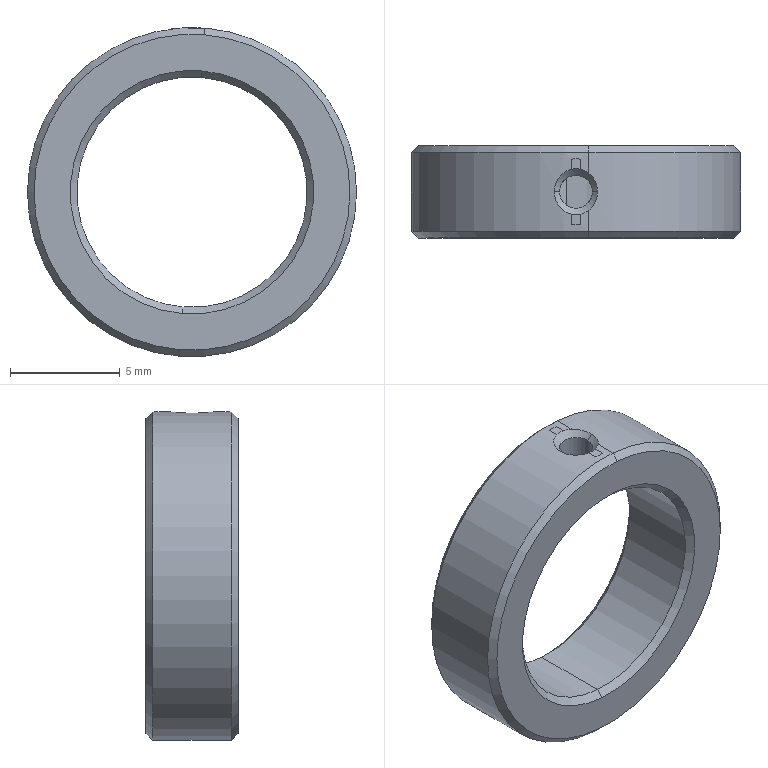Part | STEP file | 2026.6.15-Main Assembly图.sldasm-Part-197 | 1 solid | 20 faces | box 15 x 4.2 x 15 mm | volume 367.131 mm3 | cone 10 | cylinder 6 | plane 4 | commonest cylinder face diameters 1.5 x2 10.5 x2 15 x2
STEP:
#1=CARTESIAN_POINT('',(-1629.724,1422.164,3402.553));
#2=VERTEX_POINT('',#1);
#3=CARTESIAN_POINT('',(-1629.7,1422.464,3402.853));
#4=VERTEX_POINT('',#3);
#5=CARTESIAN_POINT('',(-1629.724,1422.164,3402.553));
#6=DIRECTION('',(0.0555,0.7071,0.7049));
#7=VECTOR('',#6,1000.);
#8=LINE('',#5,#7);
#9=EDGE_CURVE('',#2,#4,#8,.T.);
#10=ORIENTED_EDGE('',*,*,#9,.T.);
#11=CARTESIAN_POINT('',(-1628.876,1422.464,3413.32));
#12=VERTEX_POINT('',#11);
#13=CARTESIAN_POINT('',(-1629.288,1422.464,3408.086));
#14=DIRECTION('',(0.,1.,0.));
#15=DIRECTION('',(0.0785,0.,0.9969));
#16=AXIS2_PLACEMENT_3D('',#13,#14,#15);
#17=CIRCLE('',#16,5.25);
#18=EDGE_CURVE('',#4,#12,#17,.T.);
#19=ORIENTED_EDGE('',*,*,#18,.T.);
#20=CARTESIAN_POINT('',(-1628.853,1422.164,3413.619));
#21=VERTEX_POINT('',#20);
#22=CARTESIAN_POINT('',(-1628.853,1422.164,3413.619));
#23=DIRECTION('',(-0.0555,0.7071,-0.7049));
#24=VECTOR('',#23,1000.);
#25=LINE('',#22,#24);
#26=EDGE_CURVE('',#21,#12,#25,.T.);
#27=ORIENTED_EDGE('',*,*,#26,.F.);
#28=CARTESIAN_POINT('',(-1629.288,1422.164,3408.086));
#29=DIRECTION('',(0.,1.,0.));
#30=DIRECTION('',(0.0785,0.,0.9969));
#31=AXIS2_PLACEMENT_3D('',#28,#29,#30);
#32=CIRCLE('',#31,5.55);
#33=EDGE_CURVE('',#2,#21,#32,.T.);
#34=ORIENTED_EDGE('',*,*,#33,.F.);
#35=EDGE_LOOP('',(#10,#19,#27,#34));
#36=FACE_OUTER_BOUND('',#35,.T.);
#37=CARTESIAN_POINT('',(-1629.288,1422.164,3408.086));
#38=DIRECTION('',(0.,-1.,0.));
#39=DIRECTION('',(-0.0785,0.,-0.9969));
#40=AXIS2_PLACEMENT_3D('',#37,#38,#39);
#41=CONICAL_SURFACE('',#40,5.55,0.7854);
#42=ADVANCED_FACE('',(#36),#41,.F.);
#43=CARTESIAN_POINT('',(-1628.876,1426.064,3413.32));
#44=VERTEX_POINT('',#43);
#45=CARTESIAN_POINT('',(-1628.853,1426.364,3413.619));
#46=VERTEX_POINT('',#45);
#47=CARTESIAN_POINT('',(-1628.853,1426.364,3413.619));
#48=DIRECTION('',(0.0555,0.7071,0.7049));
#49=VECTOR('',#48,1000.);
#50=LINE('',#47,#49);
#51=EDGE_CURVE('',#44,#46,#50,.T.);
#52=ORIENTED_EDGE('',*,*,#51,.F.);
#53=CARTESIAN_POINT('',(-1629.7,1426.064,3402.853));
#54=VERTEX_POINT('',#53);
#55=CARTESIAN_POINT('',(-1629.288,1426.064,3408.086));
#56=DIRECTION('',(0.,-1.,0.));
#57=DIRECTION('',(0.0785,0.,0.9969));
#58=AXIS2_PLACEMENT_3D('',#55,#56,#57);
#59=CIRCLE('',#58,5.25);
#60=EDGE_CURVE('',#44,#54,#59,.T.);
#61=ORIENTED_EDGE('',*,*,#60,.T.);
#62=CARTESIAN_POINT('',(-1629.724,1426.364,3402.553));
#63=VERTEX_POINT('',#62);
#64=CARTESIAN_POINT('',(-1629.724,1426.364,3402.553));
#65=DIRECTION('',(-0.0555,0.7071,-0.7049));
#66=VECTOR('',#65,1000.);
#67=LINE('',#64,#66);
#68=EDGE_CURVE('',#54,#63,#67,.T.);
#69=ORIENTED_EDGE('',*,*,#68,.T.);
#70=CARTESIAN_POINT('',(-1629.288,1426.364,3408.086));
#71=DIRECTION('',(0.,1.,0.));
#72=DIRECTION('',(-0.0785,0.,-0.9969));
#73=AXIS2_PLACEMENT_3D('',#70,#71,#72);
#74=CIRCLE('',#73,5.55);
#75=EDGE_CURVE('',#63,#46,#74,.T.);
#76=ORIENTED_EDGE('',*,*,#75,.T.);
#77=EDGE_LOOP('',(#52,#61,#69,#76));
#78=FACE_OUTER_BOUND('',#77,.T.);
#79=CARTESIAN_POINT('',(-1629.288,1426.364,3408.086));
#80=DIRECTION('',(0.,1.,0.));
#81=DIRECTION('',(0.0785,0.,0.9969));
#82=AXIS2_PLACEMENT_3D('',#79,#80,#81);
#83=CONICAL_SURFACE('',#82,5.55,0.7854);
#84=ADVANCED_FACE('',(#78),#83,.F.);
#85=CARTESIAN_POINT('',(-1629.7,1404.739,3402.853));
#86=DIRECTION('',(0.,1.,0.));
#87=VECTOR('',#86,1000.);
#88=LINE('',#85,#87);
#89=EDGE_CURVE('',#4,#54,#88,.T.);
#90=ORIENTED_EDGE('',*,*,#89,.T.);
#91=ORIENTED_EDGE('',*,*,#60,.F.);
#92=CARTESIAN_POINT('',(-1628.876,1424.891,3413.32));
#93=VERTEX_POINT('',#92);
#94=CARTESIAN_POINT('',(-1628.876,1404.739,3413.32));
#95=DIRECTION('',(0.,1.,0.));
#96=VECTOR('',#95,1000.);
#97=LINE('',#94,#96);
#98=EDGE_CURVE('',#93,#44,#97,.T.);
#99=ORIENTED_EDGE('',*,*,#98,.F.);
#100=CARTESIAN_POINT('',(-1630.038,1424.264,3413.282));
#101=VERTEX_POINT('',#100);
#102=CARTESIAN_POINT('',(-1628.876,1424.891,3413.32));
#103=CARTESIAN_POINT('',(-1628.989,1424.965,3413.329));
#104=CARTESIAN_POINT('',(-1629.121,1425.008,3413.335));
#105=CARTESIAN_POINT('',(-1629.389,1425.019,3413.337));
#106=CARTESIAN_POINT('',(-1629.526,1424.988,3413.332));
#107=CARTESIAN_POINT('',(-1629.763,1424.861,3413.316));
#108=CARTESIAN_POINT('',(-1629.863,1424.765,3413.305));
#109=CARTESIAN_POINT('',(-1630.001,1424.534,3413.288));
#110=CARTESIAN_POINT('',(-1630.038,1424.4,3413.282));
#111=CARTESIAN_POINT('',(-1630.038,1424.264,3413.282));
#112=B_SPLINE_CURVE_WITH_KNOTS('',3,(#102,#103,#104,#105,#106,#107,#108,#109,#110,#111),.UNSPECIFIED.,.F.,.F.,(4,2,2,2,4),(0.,0.000402,0.000804,0.001206,0.001608),.UNSPECIFIED.);
#113=EDGE_CURVE('',#93,#101,#112,.T.);
#114=ORIENTED_EDGE('',*,*,#113,.T.);
#115=CARTESIAN_POINT('',(-1628.876,1423.638,3413.32));
#116=VERTEX_POINT('',#115);
#117=CARTESIAN_POINT('',(-1630.038,1424.264,3413.282));
#118=CARTESIAN_POINT('',(-1630.038,1424.128,3413.282));
#119=CARTESIAN_POINT('',(-1630.001,1423.995,3413.288));
#120=CARTESIAN_POINT('',(-1629.864,1423.765,3413.305));
#121=CARTESIAN_POINT('',(-1629.763,1423.668,3413.316));
#122=CARTESIAN_POINT('',(-1629.526,1423.541,3413.332));
#123=CARTESIAN_POINT('',(-1629.391,1423.509,3413.337));
#124=CARTESIAN_POINT('',(-1629.122,1423.521,3413.335));
#125=CARTESIAN_POINT('',(-1628.989,1423.563,3413.329));
#126=CARTESIAN_POINT('',(-1628.876,1423.638,3413.32));
#127=B_SPLINE_CURVE_WITH_KNOTS('',3,(#117,#118,#119,#120,#121,#122,#123,#124,#125,#126),.UNSPECIFIED.,.F.,.F.,(4,2,2,2,4),(0.,0.0004019,0.0008039,0.001206,0.001608),.UNSPECIFIED.);
#128=EDGE_CURVE('',#101,#116,#127,.T.);
#129=ORIENTED_EDGE('',*,*,#128,.T.);
#130=CARTESIAN_POINT('',(-1628.876,1404.739,3413.32));
#131=DIRECTION('',(0.,-1.,0.));
#132=VECTOR('',#131,1000.);
#133=LINE('',#130,#132);
#134=EDGE_CURVE('',#116,#12,#133,.T.);
#135=ORIENTED_EDGE('',*,*,#134,.T.);
#136=ORIENTED_EDGE('',*,*,#18,.F.);
#137=EDGE_LOOP('',(#90,#91,#99,#114,#129,#135,#136));
#138=FACE_OUTER_BOUND('',#137,.T.);
#139=CARTESIAN_POINT('',(-1629.288,1404.739,3408.086));
#140=DIRECTION('',(0.,-1.,0.));
#141=DIRECTION('',(-0.0785,0.,-0.9969));
#142=AXIS2_PLACEMENT_3D('',#139,#140,#141);
#143=CYLINDRICAL_SURFACE('',#142,5.25);
#144=ADVANCED_FACE('',(#138),#143,.F.);
#145=CARTESIAN_POINT('',(-1629.853,1422.164,3400.909));
#146=VERTEX_POINT('',#145);
#147=CARTESIAN_POINT('',(-1628.723,1422.164,3415.264));
#148=VERTEX_POINT('',#147);
#149=CARTESIAN_POINT('',(-1629.288,1422.164,3408.086));
#150=DIRECTION('',(0.,1.,0.));
#151=DIRECTION('',(-0.0785,0.,-0.9969));
#152=AXIS2_PLACEMENT_3D('',#149,#150,#151);
#153=CIRCLE('',#152,7.2);
#154=EDGE_CURVE('',#146,#148,#153,.T.);
#155=ORIENTED_EDGE('',*,*,#154,.F.);
#156=CARTESIAN_POINT('',(-1629.288,1422.164,3408.086));
#157=DIRECTION('',(0.,1.,0.));
#158=DIRECTION('',(-0.0785,0.,-0.9969));
#159=AXIS2_PLACEMENT_3D('',#156,#157,#158);
#160=CIRCLE('',#159,7.2);
#161=EDGE_CURVE('',#148,#146,#160,.T.);
#162=ORIENTED_EDGE('',*,*,#161,.F.);
#163=EDGE_LOOP('',(#155,#162));
#164=FACE_OUTER_BOUND('',#163,.T.);
#165=CARTESIAN_POINT('',(-1629.288,1422.164,3408.086));
#166=DIRECTION('',(0.,1.,0.));
#167=DIRECTION('',(0.0785,0.,0.9969));
#168=AXIS2_PLACEMENT_3D('',#165,#166,#167);
#169=CIRCLE('',#168,5.55);
#170=EDGE_CURVE('',#21,#2,#169,.T.);
#171=ORIENTED_EDGE('',*,*,#170,.T.);
#172=ORIENTED_EDGE('',*,*,#33,.T.);
#173=EDGE_LOOP('',(#171,#172));
#174=FACE_BOUND('',#173,.T.);
#175=CARTESIAN_POINT('',(-1629.288,1422.164,3408.086));
#176=DIRECTION('',(0.,-1.,0.));
#177=DIRECTION('',(0.,0.,-1.));
#178=AXIS2_PLACEMENT_3D('',#175,#176,#177);
#179=PLANE('',#178);
#180=ADVANCED_FACE('',(#164,#174),#179,.T.);
#181=CARTESIAN_POINT('',(-1628.723,1426.364,3415.264));
#182=VERTEX_POINT('',#181);
#183=CARTESIAN_POINT('',(-1629.853,1426.364,3400.909));
#184=VERTEX_POINT('',#183);
#185=CARTESIAN_POINT('',(-1629.288,1426.364,3408.086));
#186=DIRECTION('',(0.,-1.,0.));
#187=DIRECTION('',(0.0785,0.,0.9969));
#188=AXIS2_PLACEMENT_3D('',#185,#186,#187);
#189=CIRCLE('',#188,7.2);
#190=EDGE_CURVE('',#182,#184,#189,.T.);
#191=ORIENTED_EDGE('',*,*,#190,.F.);
#192=CARTESIAN_POINT('',(-1629.288,1426.364,3408.086));
#193=DIRECTION('',(0.,-1.,0.));
#194=DIRECTION('',(0.0785,0.,0.9969));
#195=AXIS2_PLACEMENT_3D('',#192,#193,#194);
#196=CIRCLE('',#195,7.2);
#197=EDGE_CURVE('',#184,#182,#196,.T.);
#198=ORIENTED_EDGE('',*,*,#197,.F.);
#199=EDGE_LOOP('',(#191,#198));
#200=FACE_OUTER_BOUND('',#199,.T.);
#201=ORIENTED_EDGE('',*,*,#75,.F.);
#202=CARTESIAN_POINT('',(-1629.288,1426.364,3408.086));
#203=DIRECTION('',(0.,1.,0.));
#204=DIRECTION('',(-0.0785,0.,-0.9969));
#205=AXIS2_PLACEMENT_3D('',#202,#203,#204);
#206=CIRCLE('',#205,5.55);
#207=EDGE_CURVE('',#46,#63,#206,.T.);
#208=ORIENTED_EDGE('',*,*,#207,.F.);
#209=EDGE_LOOP('',(#201,#208));
#210=FACE_BOUND('',#209,.T.);
#211=CARTESIAN_POINT('',(-1629.288,1426.364,3408.086));
#212=DIRECTION('',(0.,-1.,0.));
#213=DIRECTION('',(0.,0.,-1.));
#214=AXIS2_PLACEMENT_3D('',#211,#212,#213);
#215=PLANE('',#214);
#216=ADVANCED_FACE('',(#200,#210),#215,.F.);
#217=CARTESIAN_POINT('',(-1629.5,1425.29,3415.583));
#218=VERTEX_POINT('',#217);
#219=CARTESIAN_POINT('',(-1629.5,1425.749,3415.583));
#220=VERTEX_POINT('',#219);
#221=CARTESIAN_POINT('',(-1629.5,1426.364,3415.583));
#222=DIRECTION('',(0.,1.,0.));
#223=VECTOR('',#222,1000.);
#224=LINE('',#221,#223);
#225=EDGE_CURVE('',#218,#220,#224,.T.);
#226=ORIENTED_EDGE('',*,*,#225,.F.);
#227=CARTESIAN_POINT('',(-1629.076,1425.29,3415.583));
#228=VERTEX_POINT('',#227);
#229=CARTESIAN_POINT('',(-1629.288,1424.264,3415.583));
#230=DIRECTION('',(0.,0.,-1.));
#231=DIRECTION('',(1.,0.,0.));
#232=AXIS2_PLACEMENT_3D('',#229,#230,#231);
#233=CIRCLE('',#232,1.047);
#234=EDGE_CURVE('',#218,#228,#233,.T.);
#235=ORIENTED_EDGE('',*,*,#234,.T.);
#236=CARTESIAN_POINT('',(-1629.076,1425.749,3415.583));
#237=VERTEX_POINT('',#236);
#238=CARTESIAN_POINT('',(-1629.076,1426.364,3415.583));
#239=DIRECTION('',(0.,-1.,0.));
#240=VECTOR('',#239,1000.);
#241=LINE('',#238,#240);
#242=EDGE_CURVE('',#237,#228,#241,.T.);
#243=ORIENTED_EDGE('',*,*,#242,.F.);
#244=CARTESIAN_POINT('',(-1629.5,1425.749,3415.583));
#245=CARTESIAN_POINT('',(-1629.359,1425.769,3415.587));
#246=CARTESIAN_POINT('',(-1629.218,1425.769,3415.587));
#247=CARTESIAN_POINT('',(-1629.076,1425.749,3415.583));
#248=B_SPLINE_CURVE_WITH_KNOTS('',3,(#244,#245,#246,#247),.UNSPECIFIED.,.F.,.F.,(4,4),(0.,1.),.UNSPECIFIED.);
#249=EDGE_CURVE('',#220,#237,#248,.T.);
#250=ORIENTED_EDGE('',*,*,#249,.F.);
#251=EDGE_LOOP('',(#226,#235,#243,#250));
#252=FACE_OUTER_BOUND('',#251,.T.);
#253=CARTESIAN_POINT('',(-1629.288,1424.264,3415.583));
#254=DIRECTION('',(0.,0.,-1.));
#255=DIRECTION('',(1.,0.,0.));
#256=AXIS2_PLACEMENT_3D('',#253,#254,#255);
#257=PLANE('',#256);
#258=ADVANCED_FACE('',(#252),#257,.F.);
#259=CARTESIAN_POINT('',(-1629.5,1422.779,3415.583));
#260=VERTEX_POINT('',#259);
#261=CARTESIAN_POINT('',(-1629.5,1423.239,3415.583));
#262=VERTEX_POINT('',#261);
#263=CARTESIAN_POINT('',(-1629.5,1426.364,3415.583));
#264=DIRECTION('',(0.,1.,0.));
#265=VECTOR('',#264,1000.);
#266=LINE('',#263,#265);
#267=EDGE_CURVE('',#260,#262,#266,.T.);
#268=ORIENTED_EDGE('',*,*,#267,.F.);
#269=CARTESIAN_POINT('',(-1629.076,1422.779,3415.583));
#270=VERTEX_POINT('',#269);
#271=CARTESIAN_POINT('',(-1629.076,1422.779,3415.583));
#272=CARTESIAN_POINT('',(-1629.218,1422.759,3415.587));
#273=CARTESIAN_POINT('',(-1629.359,1422.759,3415.587));
#274=CARTESIAN_POINT('',(-1629.5,1422.779,3415.583));
#275=B_SPLINE_CURVE_WITH_KNOTS('',3,(#271,#272,#273,#274),.UNSPECIFIED.,.F.,.F.,(4,4),(0.,1.),.UNSPECIFIED.);
#276=EDGE_CURVE('',#270,#260,#275,.T.);
#277=ORIENTED_EDGE('',*,*,#276,.F.);
#278=CARTESIAN_POINT('',(-1629.076,1423.239,3415.583));
#279=VERTEX_POINT('',#278);
#280=CARTESIAN_POINT('',(-1629.076,1426.364,3415.583));
#281=DIRECTION('',(0.,-1.,0.));
#282=VECTOR('',#281,1000.);
#283=LINE('',#280,#282);
#284=EDGE_CURVE('',#279,#270,#283,.T.);
#285=ORIENTED_EDGE('',*,*,#284,.F.);
#286=CARTESIAN_POINT('',(-1629.288,1424.264,3415.583));
#287=DIRECTION('',(0.,0.,-1.));
#288=DIRECTION('',(1.,0.,0.));
#289=AXIS2_PLACEMENT_3D('',#286,#287,#288);
#290=CIRCLE('',#289,1.047);
#291=EDGE_CURVE('',#279,#262,#290,.T.);
#292=ORIENTED_EDGE('',*,*,#291,.T.);
#293=EDGE_LOOP('',(#268,#277,#285,#292));
#294=FACE_OUTER_BOUND('',#293,.T.);
#295=CARTESIAN_POINT('',(-1629.288,1424.264,3415.583));
#296=DIRECTION('',(0.,0.,-1.));
#297=DIRECTION('',(1.,0.,0.));
#298=AXIS2_PLACEMENT_3D('',#295,#296,#297);
#299=PLANE('',#298);
#300=ADVANCED_FACE('',(#294),#299,.F.);
#301=CARTESIAN_POINT('',(-1628.538,1424.264,3413.282));
#302=VERTEX_POINT('',#301);
#303=CARTESIAN_POINT('',(-1628.538,1424.264,3415.286));
#304=VERTEX_POINT('',#303);
#305=CARTESIAN_POINT('',(-1628.538,1424.264,3393.661));
#306=DIRECTION('',(0.,0.,1.));
#307=VECTOR('',#306,1000.);
#308=LINE('',#305,#307);
#309=EDGE_CURVE('',#302,#304,#308,.T.);
#310=ORIENTED_EDGE('',*,*,#309,.T.);
#311=CARTESIAN_POINT('',(-1630.038,1424.264,3415.286));
#312=VERTEX_POINT('',#311);
#313=CARTESIAN_POINT('',(-1629.288,1424.264,3415.286));
#314=DIRECTION('',(0.,0.,1.));
#315=DIRECTION('',(1.,0.,0.));
#316=AXIS2_PLACEMENT_3D('',#313,#314,#315);
#317=CIRCLE('',#316,0.75);
#318=EDGE_CURVE('',#304,#312,#317,.T.);
#319=ORIENTED_EDGE('',*,*,#318,.T.);
#320=CARTESIAN_POINT('',(-1630.038,1424.264,3393.661));
#321=DIRECTION('',(0.,0.,1.));
#322=VECTOR('',#321,1000.);
#323=LINE('',#320,#322);
#324=EDGE_CURVE('',#101,#312,#323,.T.);
#325=ORIENTED_EDGE('',*,*,#324,.F.);
#326=ORIENTED_EDGE('',*,*,#113,.F.);
#327=CARTESIAN_POINT('',(-1628.538,1424.264,3413.282));
#328=CARTESIAN_POINT('',(-1628.538,1424.389,3413.282));
#329=CARTESIAN_POINT('',(-1628.57,1424.512,3413.287));
#330=CARTESIAN_POINT('',(-1628.687,1424.729,3413.302));
#331=CARTESIAN_POINT('',(-1628.772,1424.822,3413.312));
#332=CARTESIAN_POINT('',(-1628.876,1424.891,3413.32));
#333=B_SPLINE_CURVE_WITH_KNOTS('',3,(#327,#328,#329,#330,#331,#332),.UNSPECIFIED.,.F.,.F.,(4,2,4),(0.,0.0003696,0.0007391),.UNSPECIFIED.);
#334=EDGE_CURVE('',#302,#93,#333,.T.);
#335=ORIENTED_EDGE('',*,*,#334,.F.);
#336=EDGE_LOOP('',(#310,#319,#325,#326,#335));
#337=FACE_OUTER_BOUND('',#336,.T.);
#338=CARTESIAN_POINT('',(-1629.288,1424.264,3393.661));
#339=DIRECTION('',(0.,0.,-1.));
#340=DIRECTION('',(1.,0.,0.));
#341=AXIS2_PLACEMENT_3D('',#338,#339,#340);
#342=CYLINDRICAL_SURFACE('',#341,0.75);
#343=ADVANCED_FACE('',(#337),#342,.F.);
#344=CARTESIAN_POINT('',(-1628.7,1422.464,3415.563));
#345=VERTEX_POINT('',#344);
#346=CARTESIAN_POINT('',(-1628.7,1422.464,3415.563));
#347=DIRECTION('',(0.0555,0.7071,0.7049));
#348=VECTOR('',#347,1000.);
#349=LINE('',#346,#348);
#350=EDGE_CURVE('',#148,#345,#349,.T.);
#351=ORIENTED_EDGE('',*,*,#350,.F.);
#352=ORIENTED_EDGE('',*,*,#161,.T.);
#353=CARTESIAN_POINT('',(-1629.877,1422.464,3400.609));
#354=VERTEX_POINT('',#353);
#355=CARTESIAN_POINT('',(-1629.877,1422.464,3400.609));
#356=DIRECTION('',(-0.0555,0.7071,-0.7049));
#357=VECTOR('',#356,1000.);
#358=LINE('',#355,#357);
#359=EDGE_CURVE('',#146,#354,#358,.T.);
#360=ORIENTED_EDGE('',*,*,#359,.T.);
#361=CARTESIAN_POINT('',(-1629.288,1422.464,3408.086));
#362=DIRECTION('',(0.,1.,0.));
#363=DIRECTION('',(-0.0785,0.,-0.9969));
#364=AXIS2_PLACEMENT_3D('',#361,#362,#363);
#365=CIRCLE('',#364,7.5);
#366=EDGE_CURVE('',#345,#354,#365,.T.);
#367=ORIENTED_EDGE('',*,*,#366,.F.);
#368=EDGE_LOOP('',(#351,#352,#360,#367));
#369=FACE_OUTER_BOUND('',#368,.T.);
#370=CARTESIAN_POINT('',(-1629.288,1422.464,3408.086));
#371=DIRECTION('',(0.,1.,0.));
#372=DIRECTION('',(0.0785,0.,0.9969));
#373=AXIS2_PLACEMENT_3D('',#370,#371,#372);
#374=CONICAL_SURFACE('',#373,7.5,0.7854);
#375=ADVANCED_FACE('',(#369),#374,.T.);
#376=CARTESIAN_POINT('',(-1629.877,1426.064,3400.609));
#377=VERTEX_POINT('',#376);
#378=CARTESIAN_POINT('',(-1629.877,1426.064,3400.609));
#379=DIRECTION('',(0.0555,0.7071,0.7049));
#380=VECTOR('',#379,1000.);
#381=LINE('',#378,#380);
#382=EDGE_CURVE('',#377,#184,#381,.T.);
#383=ORIENTED_EDGE('',*,*,#382,.T.);
#384=ORIENTED_EDGE('',*,*,#197,.T.);
#385=CARTESIAN_POINT('',(-1628.7,1426.064,3415.563));
#386=VERTEX_POINT('',#385);
#387=CARTESIAN_POINT('',(-1628.7,1426.064,3415.563));
#388=DIRECTION('',(-0.0555,0.7071,-0.7049));
#389=VECTOR('',#388,1000.);
#390=LINE('',#387,#389);
#391=EDGE_CURVE('',#386,#182,#390,.T.);
#392=ORIENTED_EDGE('',*,*,#391,.F.);
#393=CARTESIAN_POINT('',(-1629.288,1426.064,3408.086));
#394=DIRECTION('',(0.,-1.,0.));
#395=DIRECTION('',(-0.0785,0.,-0.9969));
#396=AXIS2_PLACEMENT_3D('',#393,#394,#395);
#397=CIRCLE('',#396,7.5);
#398=EDGE_CURVE('',#377,#386,#397,.T.);
#399=ORIENTED_EDGE('',*,*,#398,.F.);
#400=EDGE_LOOP('',(#383,#384,#392,#399));
#401=FACE_OUTER_BOUND('',#400,.T.);
#402=CARTESIAN_POINT('',(-1629.288,1426.064,3408.086));
#403=DIRECTION('',(0.,-1.,0.));
#404=DIRECTION('',(-0.0785,0.,-0.9969));
#405=AXIS2_PLACEMENT_3D('',#402,#403,#404);
#406=CONICAL_SURFACE('',#405,7.5,0.7854);
#407=ADVANCED_FACE('',(#401),#406,.T.);
#408=CARTESIAN_POINT('',(-1630.273,1424.264,3415.521));
#409=VERTEX_POINT('',#408);
#410=CARTESIAN_POINT('',(-1630.335,1424.264,3415.583));
#411=DIRECTION('',(-0.7071,0.,0.7071));
#412=VECTOR('',#411,1000.);
#413=LINE('',#410,#412);
#414=EDGE_CURVE('',#312,#409,#413,.T.);
#415=ORIENTED_EDGE('',*,*,#414,.F.);
#416=ORIENTED_EDGE('',*,*,#318,.F.);
#417=CARTESIAN_POINT('',(-1628.303,1424.264,3415.521));
#418=VERTEX_POINT('',#417);
#419=CARTESIAN_POINT('',(-1628.241,1424.264,3415.583));
#420=DIRECTION('',(0.7071,0.,0.7071));
#421=VECTOR('',#420,1000.);
#422=LINE('',#419,#421);
#423=EDGE_CURVE('',#304,#418,#422,.T.);
#424=ORIENTED_EDGE('',*,*,#423,.T.);
#425=CARTESIAN_POINT('',(-1628.7,1425.106,3415.563));
#426=VERTEX_POINT('',#425);
#427=CARTESIAN_POINT('',(-1628.7,1425.106,3415.563));
#428=CARTESIAN_POINT('',(-1628.447,1424.905,3415.543));
#429=CARTESIAN_POINT('',(-1628.303,1424.588,3415.521));
#430=CARTESIAN_POINT('',(-1628.303,1424.264,3415.521));
#431=B_SPLINE_CURVE_WITH_KNOTS('',3,(#427,#428,#429,#430),.UNSPECIFIED.,.F.,.F.,(4,4),(0.,0.0009599),.UNSPECIFIED.);
#432=EDGE_CURVE('',#426,#418,#431,.T.);
#433=ORIENTED_EDGE('',*,*,#432,.F.);
#434=CARTESIAN_POINT('',(-1629.076,1425.29,3415.583));
#435=CARTESIAN_POINT('',(-1628.938,1425.257,3415.579));
#436=CARTESIAN_POINT('',(-1628.81,1425.194,3415.572));
#437=CARTESIAN_POINT('',(-1628.7,1425.106,3415.563));
#438=B_SPLINE_CURVE_WITH_KNOTS('',3,(#434,#435,#436,#437),.UNSPECIFIED.,.F.,.F.,(4,4),(0.,0.0004203),.UNSPECIFIED.);
#439=EDGE_CURVE('',#228,#426,#438,.T.);
#440=ORIENTED_EDGE('',*,*,#439,.F.);
#441=ORIENTED_EDGE('',*,*,#234,.F.);
#442=CARTESIAN_POINT('',(-1630.273,1424.264,3415.521));
#443=CARTESIAN_POINT('',(-1630.273,1424.497,3415.521));
#444=CARTESIAN_POINT('',(-1630.2,1424.725,3415.532));
#445=CARTESIAN_POINT('',(-1629.927,1425.097,3415.56));
#446=CARTESIAN_POINT('',(-1629.728,1425.236,3415.577));
#447=CARTESIAN_POINT('',(-1629.5,1425.29,3415.583));
#448=B_SPLINE_CURVE_WITH_KNOTS('',3,(#442,#443,#444,#445,#446,#447),.UNSPECIFIED.,.F.,.F.,(4,2,4),(0.,0.0006893,0.001379),.UNSPECIFIED.);
#449=EDGE_CURVE('',#409,#218,#448,.T.);
#450=ORIENTED_EDGE('',*,*,#449,.F.);
#451=EDGE_LOOP('',(#415,#416,#424,#433,#440,#441,#450));
#452=FACE_OUTER_BOUND('',#451,.T.);
#453=CARTESIAN_POINT('',(-1629.288,1424.264,3415.583));
#454=DIRECTION('',(0.,0.,1.));
#455=DIRECTION('',(-1.,0.,0.));
#456=AXIS2_PLACEMENT_3D('',#453,#454,#455);
#457=CONICAL_SURFACE('',#456,1.047,0.7854);
#458=ADVANCED_FACE('',(#452),#457,.F.);
#459=CARTESIAN_POINT('',(-1628.7,1423.423,3415.563));
#460=VERTEX_POINT('',#459);
#461=CARTESIAN_POINT('',(-1628.7,1426.364,3415.563));
#462=DIRECTION('',(0.,1.,0.));
#463=VECTOR('',#462,1000.);
#464=LINE('',#461,#463);
#465=EDGE_CURVE('',#345,#460,#464,.T.);
#466=ORIENTED_EDGE('',*,*,#465,.F.);
#467=ORIENTED_EDGE('',*,*,#366,.T.);
#468=CARTESIAN_POINT('',(-1629.877,1426.364,3400.609));
#469=DIRECTION('',(0.,1.,0.));
#470=VECTOR('',#469,1000.);
#471=LINE('',#468,#470);
#472=EDGE_CURVE('',#354,#377,#471,.T.);
#473=ORIENTED_EDGE('',*,*,#472,.T.);
#474=ORIENTED_EDGE('',*,*,#398,.T.);
#475=CARTESIAN_POINT('',(-1628.7,1426.364,3415.563));
#476=DIRECTION('',(0.,1.,0.));
#477=VECTOR('',#476,1000.);
#478=LINE('',#475,#477);
#479=EDGE_CURVE('',#426,#386,#478,.T.);
#480=ORIENTED_EDGE('',*,*,#479,.F.);
#481=ORIENTED_EDGE('',*,*,#432,.T.);
#482=CARTESIAN_POINT('',(-1628.303,1424.264,3415.521));
#483=CARTESIAN_POINT('',(-1628.303,1424.183,3415.521));
#484=CARTESIAN_POINT('',(-1628.312,1424.104,3415.523));
#485=CARTESIAN_POINT('',(-1628.346,1423.948,3415.527));
#486=CARTESIAN_POINT('',(-1628.372,1423.871,3415.53));
#487=CARTESIAN_POINT('',(-1628.473,1423.654,3415.542));
#488=CARTESIAN_POINT('',(-1628.573,1423.524,3415.553));
#489=CARTESIAN_POINT('',(-1628.7,1423.423,3415.563));
#490=B_SPLINE_CURVE_WITH_KNOTS('',3,(#482,#483,#484,#485,#486,#487,#488,#489),.UNSPECIFIED.,.F.,.F.,(4,2,2,4),(0.,0.0002393,0.0004785,0.0009571),.UNSPECIFIED.);
#491=EDGE_CURVE('',#418,#460,#490,.T.);
#492=ORIENTED_EDGE('',*,*,#491,.T.);
#493=EDGE_LOOP('',(#466,#467,#473,#474,#480,#481,#492));
#494=FACE_OUTER_BOUND('',#493,.T.);
#495=CARTESIAN_POINT('',(-1629.288,1426.364,3408.086));
#496=DIRECTION('',(0.,1.,0.));
#497=DIRECTION('',(0.0785,0.,0.9969));
#498=AXIS2_PLACEMENT_3D('',#495,#496,#497);
#499=CYLINDRICAL_SURFACE('',#498,7.5);
#500=ADVANCED_FACE('',(#494),#499,.T.);
#501=CARTESIAN_POINT('',(-1629.288,1422.464,3408.086));
#502=DIRECTION('',(0.,1.,0.));
#503=DIRECTION('',(0.0785,0.,0.9969));
#504=AXIS2_PLACEMENT_3D('',#501,#502,#503);
#505=CIRCLE('',#504,5.25);
#506=EDGE_CURVE('',#12,#4,#505,.T.);
#507=ORIENTED_EDGE('',*,*,#506,.T.);
#508=ORIENTED_EDGE('',*,*,#9,.F.);
#509=ORIENTED_EDGE('',*,*,#170,.F.);
#510=ORIENTED_EDGE('',*,*,#26,.T.);
#511=EDGE_LOOP('',(#507,#508,#509,#510));
#512=FACE_OUTER_BOUND('',#511,.T.);
#513=CARTESIAN_POINT('',(-1629.288,1422.164,3408.086));
#514=DIRECTION('',(0.,-1.,0.));
#515=DIRECTION('',(-0.0785,0.,-0.9969));
#516=AXIS2_PLACEMENT_3D('',#513,#514,#515);
#517=CONICAL_SURFACE('',#516,5.55,0.7854);
#518=ADVANCED_FACE('',(#512),#517,.F.);
#519=CARTESIAN_POINT('',(-1629.288,1426.064,3408.086));
#520=DIRECTION('',(0.,-1.,0.));
#521=DIRECTION('',(0.0785,0.,0.9969));
#522=AXIS2_PLACEMENT_3D('',#519,#520,#521);
#523=CIRCLE('',#522,5.25);
#524=EDGE_CURVE('',#54,#44,#523,.T.);
#525=ORIENTED_EDGE('',*,*,#524,.T.);
#526=ORIENTED_EDGE('',*,*,#51,.T.);
#527=ORIENTED_EDGE('',*,*,#207,.T.);
#528=ORIENTED_EDGE('',*,*,#68,.F.);
#529=EDGE_LOOP('',(#525,#526,#527,#528));
#530=FACE_OUTER_BOUND('',#529,.T.);
#531=CARTESIAN_POINT('',(-1629.288,1426.364,3408.086));
#532=DIRECTION('',(0.,1.,0.));
#533=DIRECTION('',(0.0785,0.,0.9969));
#534=AXIS2_PLACEMENT_3D('',#531,#532,#533);
#535=CONICAL_SURFACE('',#534,5.55,0.7854);
#536=ADVANCED_FACE('',(#530),#535,.F.);
#537=ORIENTED_EDGE('',*,*,#524,.F.);
#538=ORIENTED_EDGE('',*,*,#89,.F.);
#539=ORIENTED_EDGE('',*,*,#506,.F.);
#540=ORIENTED_EDGE('',*,*,#134,.F.);
#541=CARTESIAN_POINT('',(-1628.876,1423.638,3413.32));
#542=CARTESIAN_POINT('',(-1628.772,1423.706,3413.312));
#543=CARTESIAN_POINT('',(-1628.687,1423.8,3413.302));
#544=CARTESIAN_POINT('',(-1628.57,1424.016,3413.287));
#545=CARTESIAN_POINT('',(-1628.538,1424.139,3413.282));
#546=CARTESIAN_POINT('',(-1628.538,1424.264,3413.282));
#547=B_SPLINE_CURVE_WITH_KNOTS('',3,(#541,#542,#543,#544,#545,#546),.UNSPECIFIED.,.F.,.F.,(4,2,4),(0.,0.0003696,0.0007391),.UNSPECIFIED.);
#548=EDGE_CURVE('',#116,#302,#547,.T.);
#549=ORIENTED_EDGE('',*,*,#548,.T.);
#550=ORIENTED_EDGE('',*,*,#334,.T.);
#551=ORIENTED_EDGE('',*,*,#98,.T.);
#552=EDGE_LOOP('',(#537,#538,#539,#540,#549,#550,#551));
#553=FACE_OUTER_BOUND('',#552,.T.);
#554=CARTESIAN_POINT('',(-1629.288,1404.739,3408.086));
#555=DIRECTION('',(0.,-1.,0.));
#556=DIRECTION('',(-0.0785,0.,-0.9969));
#557=AXIS2_PLACEMENT_3D('',#554,#555,#556);
#558=CYLINDRICAL_SURFACE('',#557,5.25);
#559=ADVANCED_FACE('',(#553),#558,.F.);
#560=CARTESIAN_POINT('',(-1629.288,1424.264,3415.286));
#561=DIRECTION('',(0.,0.,1.));
#562=DIRECTION('',(1.,0.,0.));
#563=AXIS2_PLACEMENT_3D('',#560,#561,#562);
#564=CIRCLE('',#563,0.75);
#565=EDGE_CURVE('',#312,#304,#564,.T.);
#566=ORIENTED_EDGE('',*,*,#565,.T.);
#567=ORIENTED_EDGE('',*,*,#309,.F.);
#568=ORIENTED_EDGE('',*,*,#548,.F.);
#569=ORIENTED_EDGE('',*,*,#128,.F.);
#570=ORIENTED_EDGE('',*,*,#324,.T.);
#571=EDGE_LOOP('',(#566,#567,#568,#569,#570));
#572=FACE_OUTER_BOUND('',#571,.T.);
#573=CARTESIAN_POINT('',(-1629.288,1424.264,3393.661));
#574=DIRECTION('',(0.,0.,-1.));
#575=DIRECTION('',(1.,0.,0.));
#576=AXIS2_PLACEMENT_3D('',#573,#574,#575);
#577=CYLINDRICAL_SURFACE('',#576,0.75);
#578=ADVANCED_FACE('',(#572),#577,.F.);
#579=ORIENTED_EDGE('',*,*,#154,.T.);
#580=ORIENTED_EDGE('',*,*,#350,.T.);
#581=CARTESIAN_POINT('',(-1629.288,1422.464,3408.086));
#582=DIRECTION('',(0.,1.,0.));
#583=DIRECTION('',(-0.0785,0.,-0.9969));
#584=AXIS2_PLACEMENT_3D('',#581,#582,#583);
#585=CIRCLE('',#584,7.5);
#586=EDGE_CURVE('',#354,#345,#585,.T.);
#587=ORIENTED_EDGE('',*,*,#586,.F.);
#588=ORIENTED_EDGE('',*,*,#359,.F.);
#589=EDGE_LOOP('',(#579,#580,#587,#588));
#590=FACE_OUTER_BOUND('',#589,.T.);
#591=CARTESIAN_POINT('',(-1629.288,1422.464,3408.086));
#592=DIRECTION('',(0.,1.,0.));
#593=DIRECTION('',(0.0785,0.,0.9969));
#594=AXIS2_PLACEMENT_3D('',#591,#592,#593);
#595=CONICAL_SURFACE('',#594,7.5,0.7854);
#596=ADVANCED_FACE('',(#590),#595,.T.);
#597=ORIENTED_EDGE('',*,*,#190,.T.);
#598=ORIENTED_EDGE('',*,*,#382,.F.);
#599=CARTESIAN_POINT('',(-1629.288,1426.064,3408.086));
#600=DIRECTION('',(0.,-1.,0.));
#601=DIRECTION('',(-0.0785,0.,-0.9969));
#602=AXIS2_PLACEMENT_3D('',#599,#600,#601);
#603=CIRCLE('',#602,7.5);
#604=EDGE_CURVE('',#386,#377,#603,.T.);
#605=ORIENTED_EDGE('',*,*,#604,.F.);
#606=ORIENTED_EDGE('',*,*,#391,.T.);
#607=EDGE_LOOP('',(#597,#598,#605,#606));
#608=FACE_OUTER_BOUND('',#607,.T.);
#609=CARTESIAN_POINT('',(-1629.288,1426.064,3408.086));
#610=DIRECTION('',(0.,-1.,0.));
#611=DIRECTION('',(-0.0785,0.,-0.9969));
#612=AXIS2_PLACEMENT_3D('',#609,#610,#611);
#613=CONICAL_SURFACE('',#612,7.5,0.7854);
#614=ADVANCED_FACE('',(#608),#613,.T.);
#615=ORIENTED_EDGE('',*,*,#565,.F.);
#616=ORIENTED_EDGE('',*,*,#414,.T.);
#617=CARTESIAN_POINT('',(-1629.5,1423.239,3415.583));
#618=CARTESIAN_POINT('',(-1629.727,1423.293,3415.577));
#619=CARTESIAN_POINT('',(-1629.927,1423.431,3415.56));
#620=CARTESIAN_POINT('',(-1630.2,1423.803,3415.532));
#621=CARTESIAN_POINT('',(-1630.273,1424.032,3415.521));
#622=CARTESIAN_POINT('',(-1630.273,1424.264,3415.521));
#623=B_SPLINE_CURVE_WITH_KNOTS('',3,(#617,#618,#619,#620,#621,#622),.UNSPECIFIED.,.F.,.F.,(4,2,4),(0.,0.0006899,0.00138),.UNSPECIFIED.);
#624=EDGE_CURVE('',#262,#409,#623,.T.);
#625=ORIENTED_EDGE('',*,*,#624,.F.);
#626=ORIENTED_EDGE('',*,*,#291,.F.);
#627=CARTESIAN_POINT('',(-1628.7,1423.423,3415.563));
#628=CARTESIAN_POINT('',(-1628.81,1423.335,3415.572));
#629=CARTESIAN_POINT('',(-1628.938,1423.272,3415.579));
#630=CARTESIAN_POINT('',(-1629.076,1423.239,3415.583));
#631=B_SPLINE_CURVE_WITH_KNOTS('',3,(#627,#628,#629,#630),.UNSPECIFIED.,.F.,.F.,(4,4),(0.,0.0004204),.UNSPECIFIED.);
#632=EDGE_CURVE('',#460,#279,#631,.T.);
#633=ORIENTED_EDGE('',*,*,#632,.F.);
#634=ORIENTED_EDGE('',*,*,#491,.F.);
#635=ORIENTED_EDGE('',*,*,#423,.F.);
#636=EDGE_LOOP('',(#615,#616,#625,#626,#633,#634,#635));
#637=FACE_OUTER_BOUND('',#636,.T.);
#638=CARTESIAN_POINT('',(-1629.288,1424.264,3415.583));
#639=DIRECTION('',(0.,0.,1.));
#640=DIRECTION('',(-1.,0.,0.));
#641=AXIS2_PLACEMENT_3D('',#638,#639,#640);
#642=CONICAL_SURFACE('',#641,1.047,0.7854);
#643=ADVANCED_FACE('',(#637),#642,.F.);
#644=ORIENTED_EDGE('',*,*,#586,.T.);
#645=ORIENTED_EDGE('',*,*,#465,.T.);
#646=ORIENTED_EDGE('',*,*,#632,.T.);
#647=ORIENTED_EDGE('',*,*,#284,.T.);
#648=ORIENTED_EDGE('',*,*,#276,.T.);
#649=ORIENTED_EDGE('',*,*,#267,.T.);
#650=ORIENTED_EDGE('',*,*,#624,.T.);
#651=ORIENTED_EDGE('',*,*,#449,.T.);
#652=ORIENTED_EDGE('',*,*,#225,.T.);
#653=ORIENTED_EDGE('',*,*,#249,.T.);
#654=ORIENTED_EDGE('',*,*,#242,.T.);
#655=ORIENTED_EDGE('',*,*,#439,.T.);
#656=ORIENTED_EDGE('',*,*,#479,.T.);
#657=ORIENTED_EDGE('',*,*,#604,.T.);
#658=ORIENTED_EDGE('',*,*,#472,.F.);
#659=EDGE_LOOP('',(#644,#645,#646,#647,#648,#649,#650,#651,#652,#653,#654,#655,#656,#657,#658));
#660=FACE_OUTER_BOUND('',#659,.T.);
#661=CARTESIAN_POINT('',(-1629.288,1426.364,3408.086));
#662=DIRECTION('',(0.,1.,0.));
#663=DIRECTION('',(0.0785,0.,0.9969));
#664=AXIS2_PLACEMENT_3D('',#661,#662,#663);
#665=CYLINDRICAL_SURFACE('',#664,7.5);
#666=ADVANCED_FACE('',(#660),#665,.T.);
#667=CLOSED_SHELL('',(#42,#84,#144,#180,#216,#258,#300,#343,#375,#407,#458,#500,#518,#536,#559,#578,#596,#614,#643,#666));
#668=MANIFOLD_SOLID_BREP('',#667);
#669=CARTESIAN_POINT('',(0.,0.,0.));
#670=DIRECTION('',(0.,0.,1.));
#671=DIRECTION('',(1.,0.,0.));
#672=AXIS2_PLACEMENT_3D('',#669,#670,#671);
#673=(LENGTH_UNIT()NAMED_UNIT(*)SI_UNIT(.MILLI.,.METRE.));
#674=UNCERTAINTY_MEASURE_WITH_UNIT(LENGTH_MEASURE(0.00001),#673,'','');
#675=(NAMED_UNIT(*)PLANE_ANGLE_UNIT()SI_UNIT($,.RADIAN.));
#676=(NAMED_UNIT(*)SI_UNIT($,.STERADIAN.)SOLID_ANGLE_UNIT());
#677=(GEOMETRIC_REPRESENTATION_CONTEXT(3)GLOBAL_UNCERTAINTY_ASSIGNED_CONTEXT((#674))GLOBAL_UNIT_ASSIGNED_CONTEXT((#673,#675,#676))REPRESENTATION_CONTEXT('',''));
#678=ADVANCED_BREP_SHAPE_REPRESENTATION('',(#668,#672),#677);